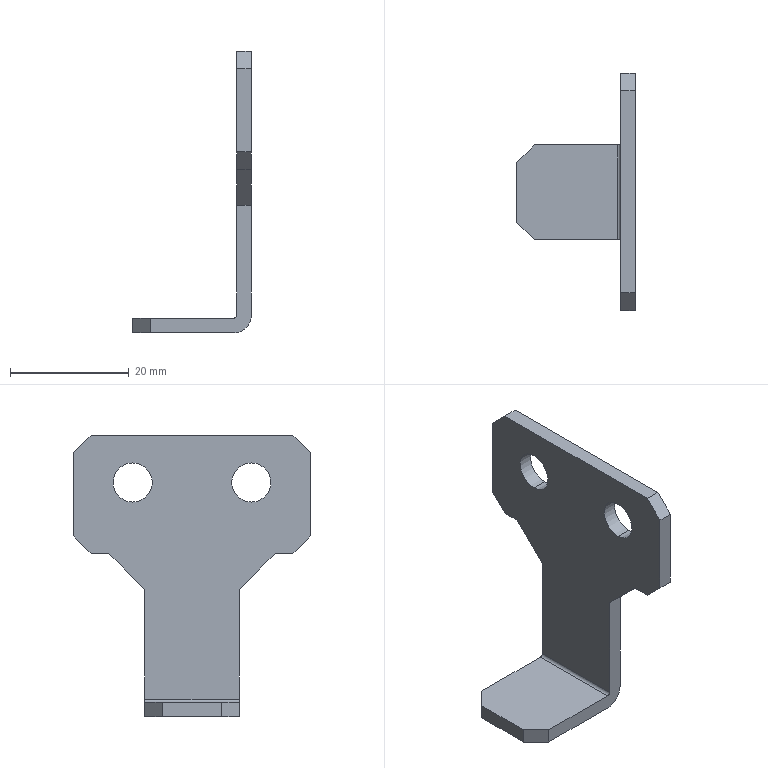Part | SolidWorks | features BaseBody 1 | 1 solid | 26 faces | box 20 x 40 x 47.5 mm | volume 3621 mm3 | plane 20 | cylinder 6 | commonest cylinder face diameters 6.6 x4 1 x1 6 x1
STEP:
#1=CARTESIAN_POINT('',(237.247,1054.806,-455.645));
#2=VERTEX_POINT('',#1);
#3=CARTESIAN_POINT('',(237.247,1054.806,-449.045));
#4=VERTEX_POINT('',#3);
#5=CARTESIAN_POINT('',(237.247,1054.806,-452.345));
#6=DIRECTION('',(-1.,0.,0.));
#7=DIRECTION('',(0.,0.,1.));
#8=AXIS2_PLACEMENT_3D('',#5,#6,#7);
#9=CIRCLE('',#8,3.3);
#10=EDGE_CURVE('',#2,#4,#9,.T.);
#11=ORIENTED_EDGE('',*,*,#10,.F.);
#12=CARTESIAN_POINT('',(234.747,1054.806,-455.645));
#13=VERTEX_POINT('',#12);
#14=CARTESIAN_POINT('',(234.747,1054.806,-455.645));
#15=DIRECTION('',(-1.,0.,0.));
#16=VECTOR('',#15,1000.);
#17=LINE('',#14,#16);
#18=EDGE_CURVE('',#2,#13,#17,.T.);
#19=ORIENTED_EDGE('',*,*,#18,.T.);
#20=CARTESIAN_POINT('',(234.747,1054.806,-449.045));
#21=VERTEX_POINT('',#20);
#22=CARTESIAN_POINT('',(234.747,1054.806,-452.345));
#23=DIRECTION('',(1.,0.,0.));
#24=DIRECTION('',(0.,0.,1.));
#25=AXIS2_PLACEMENT_3D('',#22,#23,#24);
#26=CIRCLE('',#25,3.3);
#27=EDGE_CURVE('',#21,#13,#26,.T.);
#28=ORIENTED_EDGE('',*,*,#27,.F.);
#29=CARTESIAN_POINT('',(234.747,1054.806,-449.045));
#30=DIRECTION('',(-1.,0.,0.));
#31=VECTOR('',#30,1000.);
#32=LINE('',#29,#31);
#33=EDGE_CURVE('',#4,#21,#32,.T.);
#34=ORIENTED_EDGE('',*,*,#33,.F.);
#35=EDGE_LOOP('',(#11,#19,#28,#34));
#36=FACE_OUTER_BOUND('',#35,.T.);
#37=CARTESIAN_POINT('',(234.747,1054.806,-452.345));
#38=DIRECTION('',(-1.,0.,0.));
#39=DIRECTION('',(0.,0.,1.));
#40=AXIS2_PLACEMENT_3D('',#37,#38,#39);
#41=CYLINDRICAL_SURFACE('',#40,3.3);
#42=ADVANCED_FACE('',(#36),#41,.F.);
#43=CARTESIAN_POINT('',(237.247,1034.806,-455.645));
#44=VERTEX_POINT('',#43);
#45=CARTESIAN_POINT('',(237.247,1034.806,-449.045));
#46=VERTEX_POINT('',#45);
#47=CARTESIAN_POINT('',(237.247,1034.806,-452.345));
#48=DIRECTION('',(-1.,0.,0.));
#49=DIRECTION('',(0.,0.,1.));
#50=AXIS2_PLACEMENT_3D('',#47,#48,#49);
#51=CIRCLE('',#50,3.3);
#52=EDGE_CURVE('',#44,#46,#51,.T.);
#53=ORIENTED_EDGE('',*,*,#52,.F.);
#54=CARTESIAN_POINT('',(234.747,1034.806,-455.645));
#55=VERTEX_POINT('',#54);
#56=CARTESIAN_POINT('',(234.747,1034.806,-455.645));
#57=DIRECTION('',(-1.,0.,0.));
#58=VECTOR('',#57,1000.);
#59=LINE('',#56,#58);
#60=EDGE_CURVE('',#44,#55,#59,.T.);
#61=ORIENTED_EDGE('',*,*,#60,.T.);
#62=CARTESIAN_POINT('',(234.747,1034.806,-449.045));
#63=VERTEX_POINT('',#62);
#64=CARTESIAN_POINT('',(234.747,1034.806,-452.345));
#65=DIRECTION('',(1.,0.,0.));
#66=DIRECTION('',(0.,0.,1.));
#67=AXIS2_PLACEMENT_3D('',#64,#65,#66);
#68=CIRCLE('',#67,3.3);
#69=EDGE_CURVE('',#63,#55,#68,.T.);
#70=ORIENTED_EDGE('',*,*,#69,.F.);
#71=CARTESIAN_POINT('',(234.747,1034.806,-449.045));
#72=DIRECTION('',(-1.,0.,0.));
#73=VECTOR('',#72,1000.);
#74=LINE('',#71,#73);
#75=EDGE_CURVE('',#46,#63,#74,.T.);
#76=ORIENTED_EDGE('',*,*,#75,.F.);
#77=EDGE_LOOP('',(#53,#61,#70,#76));
#78=FACE_OUTER_BOUND('',#77,.T.);
#79=CARTESIAN_POINT('',(234.747,1034.806,-452.345));
#80=DIRECTION('',(-1.,0.,0.));
#81=DIRECTION('',(0.,0.,1.));
#82=AXIS2_PLACEMENT_3D('',#79,#80,#81);
#83=CYLINDRICAL_SURFACE('',#82,3.3);
#84=ADVANCED_FACE('',(#78),#83,.F.);
#85=ORIENTED_EDGE('',*,*,#27,.T.);
#86=CARTESIAN_POINT('',(234.747,1054.806,-452.345));
#87=DIRECTION('',(1.,0.,0.));
#88=DIRECTION('',(0.,0.,1.));
#89=AXIS2_PLACEMENT_3D('',#86,#87,#88);
#90=CIRCLE('',#89,3.3);
#91=EDGE_CURVE('',#13,#21,#90,.T.);
#92=ORIENTED_EDGE('',*,*,#91,.T.);
#93=EDGE_LOOP('',(#85,#92));
#94=FACE_BOUND('',#93,.T.);
#95=ORIENTED_EDGE('',*,*,#69,.T.);
#96=CARTESIAN_POINT('',(234.747,1034.806,-452.345));
#97=DIRECTION('',(1.,0.,0.));
#98=DIRECTION('',(0.,0.,1.));
#99=AXIS2_PLACEMENT_3D('',#96,#97,#98);
#100=CIRCLE('',#99,3.3);
#101=EDGE_CURVE('',#55,#63,#100,.T.);
#102=ORIENTED_EDGE('',*,*,#101,.T.);
#103=EDGE_LOOP('',(#95,#102));
#104=FACE_BOUND('',#103,.T.);
#105=CARTESIAN_POINT('',(234.747,1052.806,-488.845));
#106=VERTEX_POINT('',#105);
#107=CARTESIAN_POINT('',(234.747,1036.806,-488.845));
#108=VERTEX_POINT('',#107);
#109=CARTESIAN_POINT('',(234.747,1044.806,-488.845));
#110=DIRECTION('',(0.,-1.,0.));
#111=VECTOR('',#110,1000.);
#112=LINE('',#109,#111);
#113=EDGE_CURVE('',#106,#108,#112,.T.);
#114=ORIENTED_EDGE('',*,*,#113,.T.);
#115=CARTESIAN_POINT('',(234.747,1036.806,-470.345));
#116=VERTEX_POINT('',#115);
#117=CARTESIAN_POINT('',(234.747,1036.806,-454.345));
#118=DIRECTION('',(0.,0.,1.));
#119=VECTOR('',#118,1000.);
#120=LINE('',#117,#119);
#121=EDGE_CURVE('',#108,#116,#120,.T.);
#122=ORIENTED_EDGE('',*,*,#121,.T.);
#123=CARTESIAN_POINT('',(234.747,1030.806,-464.345));
#124=VERTEX_POINT('',#123);
#125=CARTESIAN_POINT('',(234.747,1036.806,-470.345));
#126=DIRECTION('',(0.,-0.7071,0.7071));
#127=VECTOR('',#126,1000.);
#128=LINE('',#125,#127);
#129=EDGE_CURVE('',#116,#124,#128,.T.);
#130=ORIENTED_EDGE('',*,*,#129,.T.);
#131=CARTESIAN_POINT('',(234.747,1027.806,-464.345));
#132=VERTEX_POINT('',#131);
#133=CARTESIAN_POINT('',(234.747,1044.806,-464.345));
#134=DIRECTION('',(0.,-1.,0.));
#135=VECTOR('',#134,1000.);
#136=LINE('',#133,#135);
#137=EDGE_CURVE('',#124,#132,#136,.T.);
#138=ORIENTED_EDGE('',*,*,#137,.T.);
#139=CARTESIAN_POINT('',(234.747,1024.806,-461.345));
#140=VERTEX_POINT('',#139);
#141=CARTESIAN_POINT('',(234.747,1027.806,-464.345));
#142=DIRECTION('',(0.,-0.7071,0.7071));
#143=VECTOR('',#142,1000.);
#144=LINE('',#141,#143);
#145=EDGE_CURVE('',#132,#140,#144,.T.);
#146=ORIENTED_EDGE('',*,*,#145,.T.);
#147=CARTESIAN_POINT('',(234.747,1024.806,-447.345));
#148=VERTEX_POINT('',#147);
#149=CARTESIAN_POINT('',(234.747,1024.806,-454.345));
#150=DIRECTION('',(0.,0.,1.));
#151=VECTOR('',#150,1000.);
#152=LINE('',#149,#151);
#153=EDGE_CURVE('',#140,#148,#152,.T.);
#154=ORIENTED_EDGE('',*,*,#153,.T.);
#155=CARTESIAN_POINT('',(234.747,1027.806,-444.345));
#156=VERTEX_POINT('',#155);
#157=CARTESIAN_POINT('',(234.747,1024.806,-447.345));
#158=DIRECTION('',(0.,0.7071,0.7071));
#159=VECTOR('',#158,1000.);
#160=LINE('',#157,#159);
#161=EDGE_CURVE('',#148,#156,#160,.T.);
#162=ORIENTED_EDGE('',*,*,#161,.T.);
#163=CARTESIAN_POINT('',(234.747,1061.806,-444.345));
#164=VERTEX_POINT('',#163);
#165=CARTESIAN_POINT('',(234.747,1044.806,-444.345));
#166=DIRECTION('',(0.,1.,0.));
#167=VECTOR('',#166,1000.);
#168=LINE('',#165,#167);
#169=EDGE_CURVE('',#156,#164,#168,.T.);
#170=ORIENTED_EDGE('',*,*,#169,.T.);
#171=CARTESIAN_POINT('',(234.747,1064.806,-447.345));
#172=VERTEX_POINT('',#171);
#173=CARTESIAN_POINT('',(234.747,1061.806,-444.345));
#174=DIRECTION('',(0.,0.7071,-0.7071));
#175=VECTOR('',#174,1000.);
#176=LINE('',#173,#175);
#177=EDGE_CURVE('',#164,#172,#176,.T.);
#178=ORIENTED_EDGE('',*,*,#177,.T.);
#179=CARTESIAN_POINT('',(234.747,1064.806,-461.345));
#180=VERTEX_POINT('',#179);
#181=CARTESIAN_POINT('',(234.747,1064.806,-454.345));
#182=DIRECTION('',(0.,0.,-1.));
#183=VECTOR('',#182,1000.);
#184=LINE('',#181,#183);
#185=EDGE_CURVE('',#172,#180,#184,.T.);
#186=ORIENTED_EDGE('',*,*,#185,.T.);
#187=CARTESIAN_POINT('',(234.747,1061.806,-464.345));
#188=VERTEX_POINT('',#187);
#189=CARTESIAN_POINT('',(234.747,1064.806,-461.345));
#190=DIRECTION('',(0.,-0.7071,-0.7071));
#191=VECTOR('',#190,1000.);
#192=LINE('',#189,#191);
#193=EDGE_CURVE('',#180,#188,#192,.T.);
#194=ORIENTED_EDGE('',*,*,#193,.T.);
#195=CARTESIAN_POINT('',(234.747,1058.806,-464.345));
#196=VERTEX_POINT('',#195);
#197=CARTESIAN_POINT('',(234.747,1044.806,-464.345));
#198=DIRECTION('',(0.,-1.,0.));
#199=VECTOR('',#198,1000.);
#200=LINE('',#197,#199);
#201=EDGE_CURVE('',#188,#196,#200,.T.);
#202=ORIENTED_EDGE('',*,*,#201,.T.);
#203=CARTESIAN_POINT('',(234.747,1052.806,-470.345));
#204=VERTEX_POINT('',#203);
#205=CARTESIAN_POINT('',(234.747,1058.806,-464.345));
#206=DIRECTION('',(0.,-0.7071,-0.7071));
#207=VECTOR('',#206,1000.);
#208=LINE('',#205,#207);
#209=EDGE_CURVE('',#196,#204,#208,.T.);
#210=ORIENTED_EDGE('',*,*,#209,.T.);
#211=CARTESIAN_POINT('',(234.747,1052.806,-454.345));
#212=DIRECTION('',(0.,0.,-1.));
#213=VECTOR('',#212,1000.);
#214=LINE('',#211,#213);
#215=EDGE_CURVE('',#204,#106,#214,.T.);
#216=ORIENTED_EDGE('',*,*,#215,.T.);
#217=EDGE_LOOP('',(#114,#122,#130,#138,#146,#154,#162,#170,#178,#186,#194,#202,#210,#216));
#218=FACE_OUTER_BOUND('',#217,.T.);
#219=CARTESIAN_POINT('',(234.747,1044.806,-454.345));
#220=DIRECTION('',(-1.,0.,0.));
#221=DIRECTION('',(0.,0.,1.));
#222=AXIS2_PLACEMENT_3D('',#219,#220,#221);
#223=PLANE('',#222);
#224=ADVANCED_FACE('',(#94,#104,#218),#223,.T.);
#225=ORIENTED_EDGE('',*,*,#18,.F.);
#226=CARTESIAN_POINT('',(237.247,1054.806,-452.345));
#227=DIRECTION('',(-1.,0.,0.));
#228=DIRECTION('',(0.,0.,1.));
#229=AXIS2_PLACEMENT_3D('',#226,#227,#228);
#230=CIRCLE('',#229,3.3);
#231=EDGE_CURVE('',#4,#2,#230,.T.);
#232=ORIENTED_EDGE('',*,*,#231,.F.);
#233=ORIENTED_EDGE('',*,*,#33,.T.);
#234=ORIENTED_EDGE('',*,*,#91,.F.);
#235=EDGE_LOOP('',(#225,#232,#233,#234));
#236=FACE_OUTER_BOUND('',#235,.T.);
#237=CARTESIAN_POINT('',(234.747,1054.806,-452.345));
#238=DIRECTION('',(-1.,0.,0.));
#239=DIRECTION('',(0.,0.,1.));
#240=AXIS2_PLACEMENT_3D('',#237,#238,#239);
#241=CYLINDRICAL_SURFACE('',#240,3.3);
#242=ADVANCED_FACE('',(#236),#241,.F.);
#243=ORIENTED_EDGE('',*,*,#60,.F.);
#244=CARTESIAN_POINT('',(237.247,1034.806,-452.345));
#245=DIRECTION('',(-1.,0.,0.));
#246=DIRECTION('',(0.,0.,1.));
#247=AXIS2_PLACEMENT_3D('',#244,#245,#246);
#248=CIRCLE('',#247,3.3);
#249=EDGE_CURVE('',#46,#44,#248,.T.);
#250=ORIENTED_EDGE('',*,*,#249,.F.);
#251=ORIENTED_EDGE('',*,*,#75,.T.);
#252=ORIENTED_EDGE('',*,*,#101,.F.);
#253=EDGE_LOOP('',(#243,#250,#251,#252));
#254=FACE_OUTER_BOUND('',#253,.T.);
#255=CARTESIAN_POINT('',(234.747,1034.806,-452.345));
#256=DIRECTION('',(-1.,0.,0.));
#257=DIRECTION('',(0.,0.,1.));
#258=AXIS2_PLACEMENT_3D('',#255,#256,#257);
#259=CYLINDRICAL_SURFACE('',#258,3.3);
#260=ADVANCED_FACE('',(#254),#259,.F.);
#261=ORIENTED_EDGE('',*,*,#121,.F.);
#262=CARTESIAN_POINT('',(234.247,1036.806,-489.345));
#263=VERTEX_POINT('',#262);
#264=CARTESIAN_POINT('',(234.247,1036.806,-488.845));
#265=DIRECTION('',(0.,1.,0.));
#266=DIRECTION('',(0.,0.,-1.));
#267=AXIS2_PLACEMENT_3D('',#264,#265,#266);
#268=CIRCLE('',#267,0.5);
#269=EDGE_CURVE('',#108,#263,#268,.T.);
#270=ORIENTED_EDGE('',*,*,#269,.T.);
#271=CARTESIAN_POINT('',(220.247,1036.806,-489.345));
#272=VERTEX_POINT('',#271);
#273=CARTESIAN_POINT('',(234.747,1036.806,-489.345));
#274=DIRECTION('',(1.,0.,0.));
#275=VECTOR('',#274,1000.);
#276=LINE('',#273,#275);
#277=EDGE_CURVE('',#272,#263,#276,.T.);
#278=ORIENTED_EDGE('',*,*,#277,.F.);
#279=CARTESIAN_POINT('',(220.247,1036.806,-491.845));
#280=VERTEX_POINT('',#279);
#281=CARTESIAN_POINT('',(220.247,1036.806,-491.845));
#282=DIRECTION('',(0.,0.,1.));
#283=VECTOR('',#282,1000.);
#284=LINE('',#281,#283);
#285=EDGE_CURVE('',#280,#272,#284,.T.);
#286=ORIENTED_EDGE('',*,*,#285,.F.);
#287=CARTESIAN_POINT('',(234.247,1036.806,-491.845));
#288=VERTEX_POINT('',#287);
#289=CARTESIAN_POINT('',(217.247,1036.806,-491.845));
#290=DIRECTION('',(-1.,0.,0.));
#291=VECTOR('',#290,1000.);
#292=LINE('',#289,#291);
#293=EDGE_CURVE('',#288,#280,#292,.T.);
#294=ORIENTED_EDGE('',*,*,#293,.F.);
#295=CARTESIAN_POINT('',(237.247,1036.806,-488.845));
#296=VERTEX_POINT('',#295);
#297=CARTESIAN_POINT('',(234.247,1036.806,-488.845));
#298=DIRECTION('',(0.,1.,0.));
#299=DIRECTION('',(0.,0.,-1.));
#300=AXIS2_PLACEMENT_3D('',#297,#298,#299);
#301=CIRCLE('',#300,3.);
#302=EDGE_CURVE('',#296,#288,#301,.T.);
#303=ORIENTED_EDGE('',*,*,#302,.F.);
#304=CARTESIAN_POINT('',(237.247,1036.806,-470.345));
#305=VERTEX_POINT('',#304);
#306=CARTESIAN_POINT('',(237.247,1036.806,-488.845));
#307=DIRECTION('',(0.,0.,1.));
#308=VECTOR('',#307,1000.);
#309=LINE('',#306,#308);
#310=EDGE_CURVE('',#296,#305,#309,.T.);
#311=ORIENTED_EDGE('',*,*,#310,.T.);
#312=CARTESIAN_POINT('',(234.747,1036.806,-470.345));
#313=DIRECTION('',(-1.,0.,0.));
#314=VECTOR('',#313,1000.);
#315=LINE('',#312,#314);
#316=EDGE_CURVE('',#305,#116,#315,.T.);
#317=ORIENTED_EDGE('',*,*,#316,.T.);
#318=EDGE_LOOP('',(#261,#270,#278,#286,#294,#303,#311,#317));
#319=FACE_OUTER_BOUND('',#318,.T.);
#320=CARTESIAN_POINT('',(234.747,1036.806,-488.845));
#321=DIRECTION('',(0.,-1.,0.));
#322=DIRECTION('',(0.,0.,-1.));
#323=AXIS2_PLACEMENT_3D('',#320,#321,#322);
#324=PLANE('',#323);
#325=ADVANCED_FACE('',(#319),#324,.T.);
#326=CARTESIAN_POINT('',(234.247,1052.806,-489.345));
#327=VERTEX_POINT('',#326);
#328=CARTESIAN_POINT('',(234.247,1036.806,-489.345));
#329=DIRECTION('',(0.,1.,0.));
#330=VECTOR('',#329,1000.);
#331=LINE('',#328,#330);
#332=EDGE_CURVE('',#263,#327,#331,.T.);
#333=ORIENTED_EDGE('',*,*,#332,.F.);
#334=ORIENTED_EDGE('',*,*,#269,.F.);
#335=ORIENTED_EDGE('',*,*,#113,.F.);
#336=CARTESIAN_POINT('',(234.247,1052.806,-488.845));
#337=DIRECTION('',(0.,-1.,0.));
#338=DIRECTION('',(0.,0.,-1.));
#339=AXIS2_PLACEMENT_3D('',#336,#337,#338);
#340=CIRCLE('',#339,0.5);
#341=EDGE_CURVE('',#327,#106,#340,.T.);
#342=ORIENTED_EDGE('',*,*,#341,.F.);
#343=EDGE_LOOP('',(#333,#334,#335,#342));
#344=FACE_OUTER_BOUND('',#343,.T.);
#345=CARTESIAN_POINT('',(234.247,1036.806,-488.845));
#346=DIRECTION('',(0.,-1.,0.));
#347=DIRECTION('',(0.,0.,-1.));
#348=AXIS2_PLACEMENT_3D('',#345,#346,#347);
#349=CYLINDRICAL_SURFACE('',#348,0.5);
#350=ADVANCED_FACE('',(#344),#349,.F.);
#351=CARTESIAN_POINT('',(237.247,1052.806,-488.845));
#352=VERTEX_POINT('',#351);
#353=CARTESIAN_POINT('',(237.247,1052.806,-470.345));
#354=VERTEX_POINT('',#353);
#355=CARTESIAN_POINT('',(237.247,1052.806,-488.845));
#356=DIRECTION('',(0.,0.,1.));
#357=VECTOR('',#356,1000.);
#358=LINE('',#355,#357);
#359=EDGE_CURVE('',#352,#354,#358,.T.);
#360=ORIENTED_EDGE('',*,*,#359,.F.);
#361=CARTESIAN_POINT('',(234.247,1052.806,-491.845));
#362=VERTEX_POINT('',#361);
#363=CARTESIAN_POINT('',(234.247,1052.806,-488.845));
#364=DIRECTION('',(0.,1.,0.));
#365=DIRECTION('',(0.,0.,-1.));
#366=AXIS2_PLACEMENT_3D('',#363,#364,#365);
#367=CIRCLE('',#366,3.);
#368=EDGE_CURVE('',#352,#362,#367,.T.);
#369=ORIENTED_EDGE('',*,*,#368,.T.);
#370=CARTESIAN_POINT('',(220.247,1052.806,-491.845));
#371=VERTEX_POINT('',#370);
#372=CARTESIAN_POINT('',(234.747,1052.806,-491.845));
#373=DIRECTION('',(1.,0.,0.));
#374=VECTOR('',#373,1000.);
#375=LINE('',#372,#374);
#376=EDGE_CURVE('',#371,#362,#375,.T.);
#377=ORIENTED_EDGE('',*,*,#376,.F.);
#378=CARTESIAN_POINT('',(220.247,1052.806,-489.345));
#379=VERTEX_POINT('',#378);
#380=CARTESIAN_POINT('',(220.247,1052.806,-491.845));
#381=DIRECTION('',(0.,0.,-1.));
#382=VECTOR('',#381,1000.);
#383=LINE('',#380,#382);
#384=EDGE_CURVE('',#379,#371,#383,.T.);
#385=ORIENTED_EDGE('',*,*,#384,.F.);
#386=CARTESIAN_POINT('',(234.747,1052.806,-489.345));
#387=DIRECTION('',(-1.,0.,0.));
#388=VECTOR('',#387,1000.);
#389=LINE('',#386,#388);
#390=EDGE_CURVE('',#327,#379,#389,.T.);
#391=ORIENTED_EDGE('',*,*,#390,.F.);
#392=ORIENTED_EDGE('',*,*,#341,.T.);
#393=ORIENTED_EDGE('',*,*,#215,.F.);
#394=CARTESIAN_POINT('',(234.747,1052.806,-470.345));
#395=DIRECTION('',(-1.,0.,0.));
#396=VECTOR('',#395,1000.);
#397=LINE('',#394,#396);
#398=EDGE_CURVE('',#354,#204,#397,.T.);
#399=ORIENTED_EDGE('',*,*,#398,.F.);
#400=EDGE_LOOP('',(#360,#369,#377,#385,#391,#392,#393,#399));
#401=FACE_OUTER_BOUND('',#400,.T.);
#402=CARTESIAN_POINT('',(234.747,1052.806,-488.845));
#403=DIRECTION('',(0.,-1.,0.));
#404=DIRECTION('',(0.,0.,-1.));
#405=AXIS2_PLACEMENT_3D('',#402,#403,#404);
#406=PLANE('',#405);
#407=ADVANCED_FACE('',(#401),#406,.F.);
#408=CARTESIAN_POINT('',(237.247,1058.806,-464.345));
#409=VERTEX_POINT('',#408);
#410=CARTESIAN_POINT('',(237.247,1052.806,-470.345));
#411=DIRECTION('',(0.,0.7071,0.7071));
#412=VECTOR('',#411,1000.);
#413=LINE('',#410,#412);
#414=EDGE_CURVE('',#354,#409,#413,.T.);
#415=ORIENTED_EDGE('',*,*,#414,.F.);
#416=ORIENTED_EDGE('',*,*,#398,.T.);
#417=ORIENTED_EDGE('',*,*,#209,.F.);
#418=CARTESIAN_POINT('',(234.747,1058.806,-464.345));
#419=DIRECTION('',(-1.,0.,0.));
#420=VECTOR('',#419,1000.);
#421=LINE('',#418,#420);
#422=EDGE_CURVE('',#409,#196,#421,.T.);
#423=ORIENTED_EDGE('',*,*,#422,.F.);
#424=EDGE_LOOP('',(#415,#416,#417,#423));
#425=FACE_OUTER_BOUND('',#424,.T.);
#426=CARTESIAN_POINT('',(234.747,1052.806,-470.345));
#427=DIRECTION('',(0.,-0.7071,0.7071));
#428=DIRECTION('',(0.,-0.7071,-0.7071));
#429=AXIS2_PLACEMENT_3D('',#426,#427,#428);
#430=PLANE('',#429);
#431=ADVANCED_FACE('',(#425),#430,.F.);
#432=CARTESIAN_POINT('',(237.247,1061.806,-464.345));
#433=VERTEX_POINT('',#432);
#434=CARTESIAN_POINT('',(237.247,1061.806,-464.345));
#435=DIRECTION('',(1.,0.,0.));
#436=VECTOR('',#435,1000.);
#437=LINE('',#434,#436);
#438=EDGE_CURVE('',#188,#433,#437,.T.);
#439=ORIENTED_EDGE('',*,*,#438,.T.);
#440=CARTESIAN_POINT('',(237.247,1064.806,-464.345));
#441=DIRECTION('',(0.,-1.,0.));
#442=VECTOR('',#441,1000.);
#443=LINE('',#440,#442);
#444=EDGE_CURVE('',#433,#409,#443,.T.);
#445=ORIENTED_EDGE('',*,*,#444,.T.);
#446=ORIENTED_EDGE('',*,*,#422,.T.);
#447=ORIENTED_EDGE('',*,*,#201,.F.);
#448=EDGE_LOOP('',(#439,#445,#446,#447));
#449=FACE_OUTER_BOUND('',#448,.T.);
#450=CARTESIAN_POINT('',(237.247,1064.806,-464.345));
#451=DIRECTION('',(0.,0.,-1.));
#452=DIRECTION('',(-1.,0.,0.));
#453=AXIS2_PLACEMENT_3D('',#450,#451,#452);
#454=PLANE('',#453);
#455=ADVANCED_FACE('',(#449),#454,.T.);
#456=ORIENTED_EDGE('',*,*,#193,.F.);
#457=CARTESIAN_POINT('',(237.247,1064.806,-461.345));
#458=VERTEX_POINT('',#457);
#459=CARTESIAN_POINT('',(237.247,1064.806,-461.345));
#460=DIRECTION('',(-1.,0.,0.));
#461=VECTOR('',#460,1000.);
#462=LINE('',#459,#461);
#463=EDGE_CURVE('',#458,#180,#462,.T.);
#464=ORIENTED_EDGE('',*,*,#463,.F.);
#465=CARTESIAN_POINT('',(237.247,1064.806,-461.345));
#466=DIRECTION('',(0.,0.7071,0.7071));
#467=VECTOR('',#466,1000.);
#468=LINE('',#465,#467);
#469=EDGE_CURVE('',#433,#458,#468,.T.);
#470=ORIENTED_EDGE('',*,*,#469,.F.);
#471=ORIENTED_EDGE('',*,*,#438,.F.);
#472=EDGE_LOOP('',(#456,#464,#470,#471));
#473=FACE_OUTER_BOUND('',#472,.T.);
#474=CARTESIAN_POINT('',(237.247,1064.806,-461.345));
#475=DIRECTION('',(0.,-0.7071,0.7071));
#476=DIRECTION('',(0.,-0.7071,-0.7071));
#477=AXIS2_PLACEMENT_3D('',#474,#475,#476);
#478=PLANE('',#477);
#479=ADVANCED_FACE('',(#473),#478,.F.);
#480=CARTESIAN_POINT('',(237.247,1064.806,-447.345));
#481=VERTEX_POINT('',#480);
#482=CARTESIAN_POINT('',(237.247,1064.806,-447.345));
#483=DIRECTION('',(1.,0.,0.));
#484=VECTOR('',#483,1000.);
#485=LINE('',#482,#484);
#486=EDGE_CURVE('',#172,#481,#485,.T.);
#487=ORIENTED_EDGE('',*,*,#486,.T.);
#488=CARTESIAN_POINT('',(237.247,1064.806,-444.345));
#489=DIRECTION('',(0.,0.,-1.));
#490=VECTOR('',#489,1000.);
#491=LINE('',#488,#490);
#492=EDGE_CURVE('',#481,#458,#491,.T.);
#493=ORIENTED_EDGE('',*,*,#492,.T.);
#494=ORIENTED_EDGE('',*,*,#463,.T.);
#495=ORIENTED_EDGE('',*,*,#185,.F.);
#496=EDGE_LOOP('',(#487,#493,#494,#495));
#497=FACE_OUTER_BOUND('',#496,.T.);
#498=CARTESIAN_POINT('',(237.247,1064.806,-444.345));
#499=DIRECTION('',(0.,1.,0.));
#500=DIRECTION('',(0.,0.,1.));
#501=AXIS2_PLACEMENT_3D('',#498,#499,#500);
#502=PLANE('',#501);
#503=ADVANCED_FACE('',(#497),#502,.T.);
#504=ORIENTED_EDGE('',*,*,#177,.F.);
#505=CARTESIAN_POINT('',(237.247,1061.806,-444.345));
#506=VERTEX_POINT('',#505);
#507=CARTESIAN_POINT('',(237.247,1061.806,-444.345));
#508=DIRECTION('',(-1.,0.,0.));
#509=VECTOR('',#508,1000.);
#510=LINE('',#507,#509);
#511=EDGE_CURVE('',#506,#164,#510,.T.);
#512=ORIENTED_EDGE('',*,*,#511,.F.);
#513=CARTESIAN_POINT('',(237.247,1061.806,-444.345));
#514=DIRECTION('',(0.,-0.7071,0.7071));
#515=VECTOR('',#514,1000.);
#516=LINE('',#513,#515);
#517=EDGE_CURVE('',#481,#506,#516,.T.);
#518=ORIENTED_EDGE('',*,*,#517,.F.);
#519=ORIENTED_EDGE('',*,*,#486,.F.);
#520=EDGE_LOOP('',(#504,#512,#518,#519));
#521=FACE_OUTER_BOUND('',#520,.T.);
#522=CARTESIAN_POINT('',(237.247,1061.806,-444.345));
#523=DIRECTION('',(0.,-0.7071,-0.7071));
#524=DIRECTION('',(0.,0.7071,-0.7071));
#525=AXIS2_PLACEMENT_3D('',#522,#523,#524);
#526=PLANE('',#525);
#527=ADVANCED_FACE('',(#521),#526,.F.);
#528=ORIENTED_EDGE('',*,*,#511,.T.);
#529=ORIENTED_EDGE('',*,*,#169,.F.);
#530=CARTESIAN_POINT('',(237.247,1027.806,-444.345));
#531=VERTEX_POINT('',#530);
#532=CARTESIAN_POINT('',(237.247,1027.806,-444.345));
#533=DIRECTION('',(1.,0.,0.));
#534=VECTOR('',#533,1000.);
#535=LINE('',#532,#534);
#536=EDGE_CURVE('',#156,#531,#535,.T.);
#537=ORIENTED_EDGE('',*,*,#536,.T.);
#538=CARTESIAN_POINT('',(237.247,1064.806,-444.345));
#539=DIRECTION('',(0.,1.,0.));
#540=VECTOR('',#539,1000.);
#541=LINE('',#538,#540);
#542=EDGE_CURVE('',#531,#506,#541,.T.);
#543=ORIENTED_EDGE('',*,*,#542,.T.);
#544=EDGE_LOOP('',(#528,#529,#537,#543));
#545=FACE_OUTER_BOUND('',#544,.T.);
#546=CARTESIAN_POINT('',(237.247,1064.806,-444.345));
#547=DIRECTION('',(0.,0.,1.));
#548=DIRECTION('',(1.,0.,0.));
#549=AXIS2_PLACEMENT_3D('',#546,#547,#548);
#550=PLANE('',#549);
#551=ADVANCED_FACE('',(#545),#550,.T.);
#552=ORIENTED_EDGE('',*,*,#161,.F.);
#553=CARTESIAN_POINT('',(237.247,1024.806,-447.345));
#554=VERTEX_POINT('',#553);
#555=CARTESIAN_POINT('',(237.247,1024.806,-447.345));
#556=DIRECTION('',(-1.,0.,0.));
#557=VECTOR('',#556,1000.);
#558=LINE('',#555,#557);
#559=EDGE_CURVE('',#554,#148,#558,.T.);
#560=ORIENTED_EDGE('',*,*,#559,.F.);
#561=CARTESIAN_POINT('',(237.247,1024.806,-447.345));
#562=DIRECTION('',(0.,-0.7071,-0.7071));
#563=VECTOR('',#562,1000.);
#564=LINE('',#561,#563);
#565=EDGE_CURVE('',#531,#554,#564,.T.);
#566=ORIENTED_EDGE('',*,*,#565,.F.);
#567=ORIENTED_EDGE('',*,*,#536,.F.);
#568=EDGE_LOOP('',(#552,#560,#566,#567));
#569=FACE_OUTER_BOUND('',#568,.T.);
#570=CARTESIAN_POINT('',(237.247,1024.806,-447.345));
#571=DIRECTION('',(0.,0.7071,-0.7071));
#572=DIRECTION('',(0.,0.7071,0.7071));
#573=AXIS2_PLACEMENT_3D('',#570,#571,#572);
#574=PLANE('',#573);
#575=ADVANCED_FACE('',(#569),#574,.F.);
#576=ORIENTED_EDGE('',*,*,#559,.T.);
#577=ORIENTED_EDGE('',*,*,#153,.F.);
#578=CARTESIAN_POINT('',(237.247,1024.806,-461.345));
#579=VERTEX_POINT('',#578);
#580=CARTESIAN_POINT('',(237.247,1024.806,-461.345));
#581=DIRECTION('',(1.,0.,0.));
#582=VECTOR('',#581,1000.);
#583=LINE('',#580,#582);
#584=EDGE_CURVE('',#140,#579,#583,.T.);
#585=ORIENTED_EDGE('',*,*,#584,.T.);
#586=CARTESIAN_POINT('',(237.247,1024.806,-444.345));
#587=DIRECTION('',(0.,0.,1.));
#588=VECTOR('',#587,1000.);
#589=LINE('',#586,#588);
#590=EDGE_CURVE('',#579,#554,#589,.T.);
#591=ORIENTED_EDGE('',*,*,#590,.T.);
#592=EDGE_LOOP('',(#576,#577,#585,#591));
#593=FACE_OUTER_BOUND('',#592,.T.);
#594=CARTESIAN_POINT('',(237.247,1024.806,-444.345));
#595=DIRECTION('',(0.,-1.,0.));
#596=DIRECTION('',(0.,0.,-1.));
#597=AXIS2_PLACEMENT_3D('',#594,#595,#596);
#598=PLANE('',#597);
#599=ADVANCED_FACE('',(#593),#598,.T.);
#600=ORIENTED_EDGE('',*,*,#145,.F.);
#601=CARTESIAN_POINT('',(237.247,1027.806,-464.345));
#602=VERTEX_POINT('',#601);
#603=CARTESIAN_POINT('',(237.247,1027.806,-464.345));
#604=DIRECTION('',(-1.,0.,0.));
#605=VECTOR('',#604,1000.);
#606=LINE('',#603,#605);
#607=EDGE_CURVE('',#602,#132,#606,.T.);
#608=ORIENTED_EDGE('',*,*,#607,.F.);
#609=CARTESIAN_POINT('',(237.247,1027.806,-464.345));
#610=DIRECTION('',(0.,0.7071,-0.7071));
#611=VECTOR('',#610,1000.);
#612=LINE('',#609,#611);
#613=EDGE_CURVE('',#579,#602,#612,.T.);
#614=ORIENTED_EDGE('',*,*,#613,.F.);
#615=ORIENTED_EDGE('',*,*,#584,.F.);
#616=EDGE_LOOP('',(#600,#608,#614,#615));
#617=FACE_OUTER_BOUND('',#616,.T.);
#618=CARTESIAN_POINT('',(237.247,1027.806,-464.345));
#619=DIRECTION('',(0.,0.7071,0.7071));
#620=DIRECTION('',(0.,-0.7071,0.7071));
#621=AXIS2_PLACEMENT_3D('',#618,#619,#620);
#622=PLANE('',#621);
#623=ADVANCED_FACE('',(#617),#622,.F.);
#624=ORIENTED_EDGE('',*,*,#607,.T.);
#625=ORIENTED_EDGE('',*,*,#137,.F.);
#626=CARTESIAN_POINT('',(237.247,1030.806,-464.345));
#627=VERTEX_POINT('',#626);
#628=CARTESIAN_POINT('',(237.247,1030.806,-464.345));
#629=DIRECTION('',(1.,0.,0.));
#630=VECTOR('',#629,1000.);
#631=LINE('',#628,#630);
#632=EDGE_CURVE('',#124,#627,#631,.T.);
#633=ORIENTED_EDGE('',*,*,#632,.T.);
#634=CARTESIAN_POINT('',(237.247,1064.806,-464.345));
#635=DIRECTION('',(0.,-1.,0.));
#636=VECTOR('',#635,1000.);
#637=LINE('',#634,#636);
#638=EDGE_CURVE('',#627,#602,#637,.T.);
#639=ORIENTED_EDGE('',*,*,#638,.T.);
#640=EDGE_LOOP('',(#624,#625,#633,#639));
#641=FACE_OUTER_BOUND('',#640,.T.);
#642=CARTESIAN_POINT('',(237.247,1064.806,-464.345));
#643=DIRECTION('',(0.,0.,-1.));
#644=DIRECTION('',(-1.,0.,0.));
#645=AXIS2_PLACEMENT_3D('',#642,#643,#644);
#646=PLANE('',#645);
#647=ADVANCED_FACE('',(#641),#646,.T.);
#648=ORIENTED_EDGE('',*,*,#632,.F.);
#649=ORIENTED_EDGE('',*,*,#129,.F.);
#650=ORIENTED_EDGE('',*,*,#316,.F.);
#651=CARTESIAN_POINT('',(237.247,1030.806,-464.345));
#652=DIRECTION('',(0.,-0.7071,0.7071));
#653=VECTOR('',#652,1000.);
#654=LINE('',#651,#653);
#655=EDGE_CURVE('',#305,#627,#654,.T.);
#656=ORIENTED_EDGE('',*,*,#655,.T.);
#657=EDGE_LOOP('',(#648,#649,#650,#656));
#658=FACE_OUTER_BOUND('',#657,.T.);
#659=CARTESIAN_POINT('',(237.247,1030.806,-464.345));
#660=DIRECTION('',(0.,-0.7071,-0.7071));
#661=DIRECTION('',(0.,0.7071,-0.7071));
#662=AXIS2_PLACEMENT_3D('',#659,#660,#661);
#663=PLANE('',#662);
#664=ADVANCED_FACE('',(#658),#663,.T.);
#665=ORIENTED_EDGE('',*,*,#231,.T.);
#666=ORIENTED_EDGE('',*,*,#10,.T.);
#667=EDGE_LOOP('',(#665,#666));
#668=FACE_BOUND('',#667,.T.);
#669=ORIENTED_EDGE('',*,*,#249,.T.);
#670=ORIENTED_EDGE('',*,*,#52,.T.);
#671=EDGE_LOOP('',(#669,#670));
#672=FACE_BOUND('',#671,.T.);
#673=ORIENTED_EDGE('',*,*,#638,.F.);
#674=ORIENTED_EDGE('',*,*,#655,.F.);
#675=ORIENTED_EDGE('',*,*,#310,.F.);
#676=CARTESIAN_POINT('',(237.247,1044.806,-488.845));
#677=DIRECTION('',(0.,-1.,0.));
#678=VECTOR('',#677,1000.);
#679=LINE('',#676,#678);
#680=EDGE_CURVE('',#352,#296,#679,.T.);
#681=ORIENTED_EDGE('',*,*,#680,.F.);
#682=ORIENTED_EDGE('',*,*,#359,.T.);
#683=ORIENTED_EDGE('',*,*,#414,.T.);
#684=ORIENTED_EDGE('',*,*,#444,.F.);
#685=ORIENTED_EDGE('',*,*,#469,.T.);
#686=ORIENTED_EDGE('',*,*,#492,.F.);
#687=ORIENTED_EDGE('',*,*,#517,.T.);
#688=ORIENTED_EDGE('',*,*,#542,.F.);
#689=ORIENTED_EDGE('',*,*,#565,.T.);
#690=ORIENTED_EDGE('',*,*,#590,.F.);
#691=ORIENTED_EDGE('',*,*,#613,.T.);
#692=EDGE_LOOP('',(#673,#674,#675,#681,#682,#683,#684,#685,#686,#687,#688,#689,#690,#691));
#693=FACE_OUTER_BOUND('',#692,.T.);
#694=CARTESIAN_POINT('',(237.247,1044.806,-454.345));
#695=DIRECTION('',(-1.,0.,0.));
#696=DIRECTION('',(0.,0.,1.));
#697=AXIS2_PLACEMENT_3D('',#694,#695,#696);
#698=PLANE('',#697);
#699=ADVANCED_FACE('',(#668,#672,#693),#698,.F.);
#700=ORIENTED_EDGE('',*,*,#332,.T.);
#701=ORIENTED_EDGE('',*,*,#390,.T.);
#702=CARTESIAN_POINT('',(217.247,1049.806,-489.345));
#703=VERTEX_POINT('',#702);
#704=CARTESIAN_POINT('',(220.247,1052.806,-489.345));
#705=DIRECTION('',(-0.7071,-0.7071,0.));
#706=VECTOR('',#705,1000.);
#707=LINE('',#704,#706);
#708=EDGE_CURVE('',#379,#703,#707,.T.);
#709=ORIENTED_EDGE('',*,*,#708,.T.);
#710=CARTESIAN_POINT('',(217.247,1039.806,-489.345));
#711=VERTEX_POINT('',#710);
#712=CARTESIAN_POINT('',(217.247,1044.806,-489.345));
#713=DIRECTION('',(0.,-1.,0.));
#714=VECTOR('',#713,1000.);
#715=LINE('',#712,#714);
#716=EDGE_CURVE('',#703,#711,#715,.T.);
#717=ORIENTED_EDGE('',*,*,#716,.T.);
#718=CARTESIAN_POINT('',(217.247,1039.806,-489.345));
#719=DIRECTION('',(0.7071,-0.7071,0.));
#720=VECTOR('',#719,1000.);
#721=LINE('',#718,#720);
#722=EDGE_CURVE('',#711,#272,#721,.T.);
#723=ORIENTED_EDGE('',*,*,#722,.T.);
#724=ORIENTED_EDGE('',*,*,#277,.T.);
#725=EDGE_LOOP('',(#700,#701,#709,#717,#723,#724));
#726=FACE_OUTER_BOUND('',#725,.T.);
#727=CARTESIAN_POINT('',(234.747,1044.806,-489.345));
#728=DIRECTION('',(0.,0.,1.));
#729=DIRECTION('',(1.,0.,0.));
#730=AXIS2_PLACEMENT_3D('',#727,#728,#729);
#731=PLANE('',#730);
#732=ADVANCED_FACE('',(#726),#731,.T.);
#733=ORIENTED_EDGE('',*,*,#368,.F.);
#734=ORIENTED_EDGE('',*,*,#680,.T.);
#735=ORIENTED_EDGE('',*,*,#302,.T.);
#736=CARTESIAN_POINT('',(234.247,1036.806,-491.845));
#737=DIRECTION('',(0.,1.,0.));
#738=VECTOR('',#737,1000.);
#739=LINE('',#736,#738);
#740=EDGE_CURVE('',#288,#362,#739,.T.);
#741=ORIENTED_EDGE('',*,*,#740,.T.);
#742=EDGE_LOOP('',(#733,#734,#735,#741));
#743=FACE_OUTER_BOUND('',#742,.T.);
#744=CARTESIAN_POINT('',(234.247,1036.806,-488.845));
#745=DIRECTION('',(0.,-1.,0.));
#746=DIRECTION('',(0.,0.,-1.));
#747=AXIS2_PLACEMENT_3D('',#744,#745,#746);
#748=CYLINDRICAL_SURFACE('',#747,3.);
#749=ADVANCED_FACE('',(#743),#748,.T.);
#750=ORIENTED_EDGE('',*,*,#722,.F.);
#751=CARTESIAN_POINT('',(217.247,1039.806,-491.845));
#752=VERTEX_POINT('',#751);
#753=CARTESIAN_POINT('',(217.247,1039.806,-491.845));
#754=DIRECTION('',(0.,0.,1.));
#755=VECTOR('',#754,1000.);
#756=LINE('',#753,#755);
#757=EDGE_CURVE('',#752,#711,#756,.T.);
#758=ORIENTED_EDGE('',*,*,#757,.F.);
#759=CARTESIAN_POINT('',(217.247,1039.806,-491.845));
#760=DIRECTION('',(-0.7071,0.7071,0.));
#761=VECTOR('',#760,1000.);
#762=LINE('',#759,#761);
#763=EDGE_CURVE('',#280,#752,#762,.T.);
#764=ORIENTED_EDGE('',*,*,#763,.F.);
#765=ORIENTED_EDGE('',*,*,#285,.T.);
#766=EDGE_LOOP('',(#750,#758,#764,#765));
#767=FACE_OUTER_BOUND('',#766,.T.);
#768=CARTESIAN_POINT('',(217.247,1039.806,-491.845));
#769=DIRECTION('',(0.7071,0.7071,0.));
#770=DIRECTION('',(-0.7071,0.7071,0.));
#771=AXIS2_PLACEMENT_3D('',#768,#769,#770);
#772=PLANE('',#771);
#773=ADVANCED_FACE('',(#767),#772,.F.);
#774=CARTESIAN_POINT('',(217.247,1049.806,-491.845));
#775=VERTEX_POINT('',#774);
#776=CARTESIAN_POINT('',(217.247,1052.806,-491.845));
#777=DIRECTION('',(0.,1.,0.));
#778=VECTOR('',#777,1000.);
#779=LINE('',#776,#778);
#780=EDGE_CURVE('',#752,#775,#779,.T.);
#781=ORIENTED_EDGE('',*,*,#780,.F.);
#782=ORIENTED_EDGE('',*,*,#757,.T.);
#783=ORIENTED_EDGE('',*,*,#716,.F.);
#784=CARTESIAN_POINT('',(217.247,1049.806,-491.845));
#785=DIRECTION('',(0.,0.,1.));
#786=VECTOR('',#785,1000.);
#787=LINE('',#784,#786);
#788=EDGE_CURVE('',#775,#703,#787,.T.);
#789=ORIENTED_EDGE('',*,*,#788,.F.);
#790=EDGE_LOOP('',(#781,#782,#783,#789));
#791=FACE_OUTER_BOUND('',#790,.T.);
#792=CARTESIAN_POINT('',(217.247,1052.806,-491.845));
#793=DIRECTION('',(1.,0.,0.));
#794=DIRECTION('',(0.,0.,-1.));
#795=AXIS2_PLACEMENT_3D('',#792,#793,#794);
#796=PLANE('',#795);
#797=ADVANCED_FACE('',(#791),#796,.F.);
#798=ORIENTED_EDGE('',*,*,#708,.F.);
#799=ORIENTED_EDGE('',*,*,#384,.T.);
#800=CARTESIAN_POINT('',(220.247,1052.806,-491.845));
#801=DIRECTION('',(0.7071,0.7071,0.));
#802=VECTOR('',#801,1000.);
#803=LINE('',#800,#802);
#804=EDGE_CURVE('',#775,#371,#803,.T.);
#805=ORIENTED_EDGE('',*,*,#804,.F.);
#806=ORIENTED_EDGE('',*,*,#788,.T.);
#807=EDGE_LOOP('',(#798,#799,#805,#806));
#808=FACE_OUTER_BOUND('',#807,.T.);
#809=CARTESIAN_POINT('',(220.247,1052.806,-491.845));
#810=DIRECTION('',(0.7071,-0.7071,0.));
#811=DIRECTION('',(0.7071,0.7071,0.));
#812=AXIS2_PLACEMENT_3D('',#809,#810,#811);
#813=PLANE('',#812);
#814=ADVANCED_FACE('',(#808),#813,.F.);
#815=ORIENTED_EDGE('',*,*,#376,.T.);
#816=ORIENTED_EDGE('',*,*,#740,.F.);
#817=ORIENTED_EDGE('',*,*,#293,.T.);
#818=ORIENTED_EDGE('',*,*,#763,.T.);
#819=ORIENTED_EDGE('',*,*,#780,.T.);
#820=ORIENTED_EDGE('',*,*,#804,.T.);
#821=EDGE_LOOP('',(#815,#816,#817,#818,#819,#820));
#822=FACE_OUTER_BOUND('',#821,.T.);
#823=CARTESIAN_POINT('',(234.747,1044.806,-491.845));
#824=DIRECTION('',(0.,0.,1.));
#825=DIRECTION('',(1.,0.,0.));
#826=AXIS2_PLACEMENT_3D('',#823,#824,#825);
#827=PLANE('',#826);
#828=ADVANCED_FACE('',(#822),#827,.F.);
#829=CLOSED_SHELL('',(#42,#84,#224,#242,#260,#325,#350,#407,#431,#455,#479,#503,#527,#551,#575,#599,#623,#647,#664,#699,#732,#749,#773,#797,#814,#828));
#830=MANIFOLD_SOLID_BREP('',#829);
#831=CARTESIAN_POINT('',(0.,0.,0.));
#832=DIRECTION('',(0.,0.,1.));
#833=DIRECTION('',(1.,0.,0.));
#834=AXIS2_PLACEMENT_3D('',#831,#832,#833);
#835=(LENGTH_UNIT()NAMED_UNIT(*)SI_UNIT(.MILLI.,.METRE.));
#836=UNCERTAINTY_MEASURE_WITH_UNIT(LENGTH_MEASURE(0.00001),#835,'','');
#837=(NAMED_UNIT(*)PLANE_ANGLE_UNIT()SI_UNIT($,.RADIAN.));
#838=(NAMED_UNIT(*)SI_UNIT($,.STERADIAN.)SOLID_ANGLE_UNIT());
#839=(GEOMETRIC_REPRESENTATION_CONTEXT(3)GLOBAL_UNCERTAINTY_ASSIGNED_CONTEXT((#836))GLOBAL_UNIT_ASSIGNED_CONTEXT((#835,#837,#838))REPRESENTATION_CONTEXT('',''));
#840=ADVANCED_BREP_SHAPE_REPRESENTATION('',(#830,#834),#839);